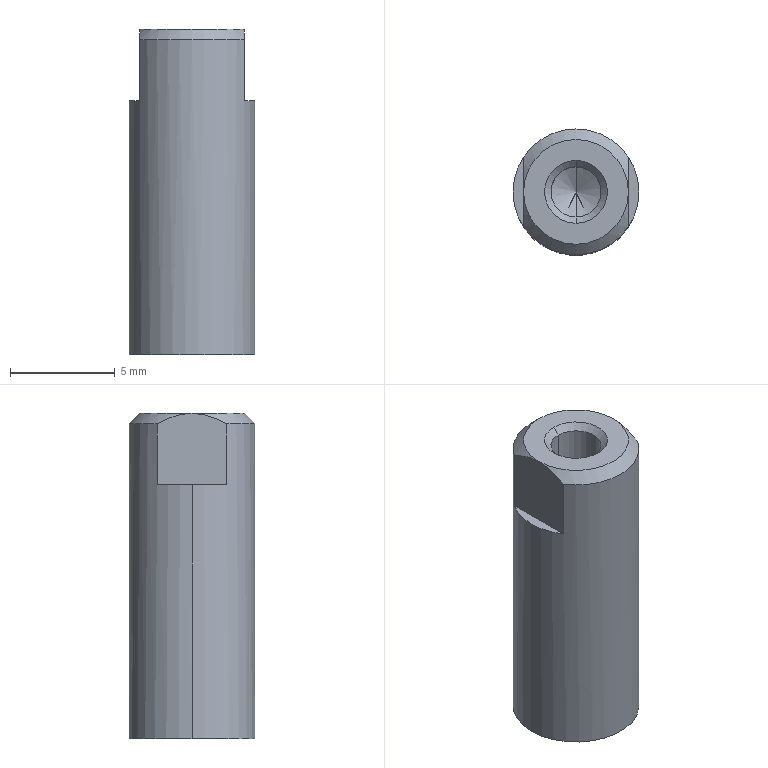Part | STEP file | 4 | 1 solid | 16 faces | box 6 x 6 x 15.5 mm | volume 398.486 mm3 | cone 6 | plane 6 | cylinder 4 | commonest cylinder face diameters 2.39 x2 6 x2
STEP:
#1=CARTESIAN_POINT('',(0.,0.,0.));
#2=DIRECTION('',(0.,0.,1.));
#3=DIRECTION('',(1.,0.,0.));
#4=AXIS2_PLACEMENT_3D('',#1,#2,#3);
#5=CARTESIAN_POINT('',(2.5,1.658,0.1));
#6=VERTEX_POINT('',#5);
#7=CARTESIAN_POINT('',(3.,0.,0.1));
#8=VERTEX_POINT('',#7);
#9=CARTESIAN_POINT('',(0.,0.,0.1));
#10=DIRECTION('',(0.,0.,-1.));
#11=DIRECTION('',(-1.,0.,0.));
#12=AXIS2_PLACEMENT_3D('',#9,#10,#11);
#13=CIRCLE('',#12,3.);
#14=CARTESIAN_POINT('',(0.,0.,-4.5));
#15=DIRECTION('',(0.,0.,-1.));
#16=DIRECTION('',(-1.,0.,0.));
#17=AXIS2_PLACEMENT_3D('',#14,#15,#16);
#18=CYLINDRICAL_SURFACE('',#17,3.);
#19=CARTESIAN_POINT('',(0.,-4.6));
#20=DIRECTION('',(1.,0.));
#21=VECTOR('',#20,1.);
#22=LINE('',#19,#21);
#23=(GEOMETRIC_REPRESENTATION_CONTEXT(2)PARAMETRIC_REPRESENTATION_CONTEXT()REPRESENTATION_CONTEXT('',''));
#24=DEFINITIONAL_REPRESENTATION('',(#22),#23);
#25=PCURVE('',#18,#24);
#26=CARTESIAN_POINT('',(0.,0.,0.1));
#27=DIRECTION('',(0.,0.,1.));
#28=DIRECTION('',(1.,0.,0.));
#29=AXIS2_PLACEMENT_3D('',#26,#27,#28);
#30=PLANE('',#29);
#31=CARTESIAN_POINT('',(-3.,0.));
#32=CARTESIAN_POINT('',(-3.,5.196));
#33=CARTESIAN_POINT('',(1.5,2.598));
#34=CARTESIAN_POINT('',(6.,0.));
#35=CARTESIAN_POINT('',(1.5,-2.598));
#36=CARTESIAN_POINT('',(-3.,-5.196));
#37=CARTESIAN_POINT('',(-3.,0.));
#38=(BOUNDED_CURVE()B_SPLINE_CURVE(2,(#31,#32,#33,#34,#35,#36,#37),.UNSPECIFIED.,.T.,.F.)B_SPLINE_CURVE_WITH_KNOTS((1,2,2,2,2,1),(-2.094,0.,2.094,4.189,6.283,8.378),.UNSPECIFIED.)CURVE()GEOMETRIC_REPRESENTATION_ITEM()RATIONAL_B_SPLINE_CURVE((1.,0.5,1.,0.5,1.,0.5,1.))REPRESENTATION_ITEM(''));
#39=(GEOMETRIC_REPRESENTATION_CONTEXT(2)PARAMETRIC_REPRESENTATION_CONTEXT()REPRESENTATION_CONTEXT('',''));
#40=DEFINITIONAL_REPRESENTATION('',(#38),#39);
#41=PCURVE('',#30,#40);
#42=SURFACE_CURVE('',#13,(#25,#41),.PCURVE_S1.);
#43=EDGE_CURVE('',#6,#8,#42,.T.);
#44=ORIENTED_EDGE('',*,*,#43,.T.);
#45=CARTESIAN_POINT('',(3.,0.,-12.));
#46=VERTEX_POINT('',#45);
#47=CARTESIAN_POINT('',(3.,0.,-4.5));
#48=DIRECTION('',(0.,0.,-1.));
#49=VECTOR('',#48,1.);
#50=LINE('',#47,#49);
#51=CARTESIAN_POINT('',(3.142,0.));
#52=DIRECTION('',(0.,1.));
#53=VECTOR('',#52,1.);
#54=LINE('',#51,#53);
#55=(GEOMETRIC_REPRESENTATION_CONTEXT(2)PARAMETRIC_REPRESENTATION_CONTEXT()REPRESENTATION_CONTEXT('',''));
#56=DEFINITIONAL_REPRESENTATION('',(#54),#55);
#57=PCURVE('',#18,#56);
#58=CARTESIAN_POINT('',(0.,0.,-4.5));
#59=DIRECTION('',(0.,0.,-1.));
#60=DIRECTION('',(-1.,0.,0.));
#61=AXIS2_PLACEMENT_3D('',#58,#59,#60);
#62=CYLINDRICAL_SURFACE('',#61,3.);
#63=CARTESIAN_POINT('',(3.142,0.));
#64=DIRECTION('',(0.,1.));
#65=VECTOR('',#64,1.);
#66=LINE('',#63,#65);
#67=(GEOMETRIC_REPRESENTATION_CONTEXT(2)PARAMETRIC_REPRESENTATION_CONTEXT()REPRESENTATION_CONTEXT('',''));
#68=DEFINITIONAL_REPRESENTATION('',(#66),#67);
#69=PCURVE('',#62,#68);
#70=SURFACE_CURVE('',#50,(#57,#69),.PCURVE_S1.);
#71=EDGE_CURVE('',#8,#46,#70,.T.);
#72=ORIENTED_EDGE('',*,*,#71,.T.);
#73=CARTESIAN_POINT('',(-3.,0.,-12.));
#74=VERTEX_POINT('',#73);
#75=CARTESIAN_POINT('',(0.,0.,-12.));
#76=DIRECTION('',(0.,0.,1.));
#77=DIRECTION('',(-1.,0.,0.));
#78=AXIS2_PLACEMENT_3D('',#75,#76,#77);
#79=CIRCLE('',#78,3.);
#80=CARTESIAN_POINT('',(6.283,7.5));
#81=DIRECTION('',(-1.,0.));
#82=VECTOR('',#81,1.);
#83=LINE('',#80,#82);
#84=(GEOMETRIC_REPRESENTATION_CONTEXT(2)PARAMETRIC_REPRESENTATION_CONTEXT()REPRESENTATION_CONTEXT('',''));
#85=DEFINITIONAL_REPRESENTATION('',(#83),#84);
#86=PCURVE('',#18,#85);
#87=CARTESIAN_POINT('',(0.,1.5,-12.));
#88=DIRECTION('',(0.,0.,-1.));
#89=DIRECTION('',(-1.,0.,0.));
#90=AXIS2_PLACEMENT_3D('',#87,#88,#89);
#91=PLANE('',#90);
#92=CARTESIAN_POINT('',(3.,-1.5));
#93=CARTESIAN_POINT('',(3.,-6.696));
#94=CARTESIAN_POINT('',(-1.5,-4.098));
#95=CARTESIAN_POINT('',(-6.,-1.5));
#96=CARTESIAN_POINT('',(-1.5,1.098));
#97=CARTESIAN_POINT('',(3.,3.696));
#98=CARTESIAN_POINT('',(3.,-1.5));
#99=(BOUNDED_CURVE()B_SPLINE_CURVE(2,(#92,#93,#94,#95,#96,#97,#98),.UNSPECIFIED.,.T.,.F.)B_SPLINE_CURVE_WITH_KNOTS((1,2,2,2,2,1),(-2.094,0.,2.094,4.189,6.283,8.378),.UNSPECIFIED.)CURVE()GEOMETRIC_REPRESENTATION_ITEM()RATIONAL_B_SPLINE_CURVE((1.,0.5,1.,0.5,1.,0.5,1.))REPRESENTATION_ITEM(''));
#100=(GEOMETRIC_REPRESENTATION_CONTEXT(2)PARAMETRIC_REPRESENTATION_CONTEXT()REPRESENTATION_CONTEXT('',''));
#101=DEFINITIONAL_REPRESENTATION('',(#99),#100);
#102=PCURVE('',#91,#101);
#103=SURFACE_CURVE('',#79,(#86,#102),.PCURVE_S1.);
#104=EDGE_CURVE('',#46,#74,#103,.T.);
#105=ORIENTED_EDGE('',*,*,#104,.T.);
#106=CARTESIAN_POINT('',(-3.,0.,0.1));
#107=VERTEX_POINT('',#106);
#108=CARTESIAN_POINT('',(-3.,0.,-4.5));
#109=DIRECTION('',(0.,0.,-1.));
#110=VECTOR('',#109,1.);
#111=LINE('',#108,#110);
#112=CARTESIAN_POINT('',(0.,0.));
#113=DIRECTION('',(0.,1.));
#114=VECTOR('',#113,1.);
#115=LINE('',#112,#114);
#116=(GEOMETRIC_REPRESENTATION_CONTEXT(2)PARAMETRIC_REPRESENTATION_CONTEXT()REPRESENTATION_CONTEXT('',''));
#117=DEFINITIONAL_REPRESENTATION('',(#115),#116);
#118=PCURVE('',#18,#117);
#119=CARTESIAN_POINT('',(6.283,0.));
#120=DIRECTION('',(0.,1.));
#121=VECTOR('',#120,1.);
#122=LINE('',#119,#121);
#123=(GEOMETRIC_REPRESENTATION_CONTEXT(2)PARAMETRIC_REPRESENTATION_CONTEXT()REPRESENTATION_CONTEXT('',''));
#124=DEFINITIONAL_REPRESENTATION('',(#122),#123);
#125=PCURVE('',#62,#124);
#126=SURFACE_CURVE('',#111,(#118,#125),.PCURVE_S1.);
#127=EDGE_CURVE('',#107,#74,#126,.T.);
#128=ORIENTED_EDGE('',*,*,#127,.F.);
#129=CARTESIAN_POINT('',(-2.5,1.658,0.1));
#130=VERTEX_POINT('',#129);
#131=CARTESIAN_POINT('',(0.,0.,0.1));
#132=DIRECTION('',(0.,0.,-1.));
#133=DIRECTION('',(-1.,0.,0.));
#134=AXIS2_PLACEMENT_3D('',#131,#132,#133);
#135=CIRCLE('',#134,3.);
#136=CARTESIAN_POINT('',(0.,-4.6));
#137=DIRECTION('',(1.,0.));
#138=VECTOR('',#137,1.);
#139=LINE('',#136,#138);
#140=(GEOMETRIC_REPRESENTATION_CONTEXT(2)PARAMETRIC_REPRESENTATION_CONTEXT()REPRESENTATION_CONTEXT('',''));
#141=DEFINITIONAL_REPRESENTATION('',(#139),#140);
#142=PCURVE('',#18,#141);
#143=CARTESIAN_POINT('',(0.,0.,0.1));
#144=DIRECTION('',(0.,0.,1.));
#145=DIRECTION('',(1.,0.,0.));
#146=AXIS2_PLACEMENT_3D('',#143,#144,#145);
#147=PLANE('',#146);
#148=CARTESIAN_POINT('',(-3.,0.));
#149=CARTESIAN_POINT('',(-3.,5.196));
#150=CARTESIAN_POINT('',(1.5,2.598));
#151=CARTESIAN_POINT('',(6.,0.));
#152=CARTESIAN_POINT('',(1.5,-2.598));
#153=CARTESIAN_POINT('',(-3.,-5.196));
#154=CARTESIAN_POINT('',(-3.,0.));
#155=(BOUNDED_CURVE()B_SPLINE_CURVE(2,(#148,#149,#150,#151,#152,#153,#154),.UNSPECIFIED.,.T.,.F.)B_SPLINE_CURVE_WITH_KNOTS((1,2,2,2,2,1),(-2.094,0.,2.094,4.189,6.283,8.378),.UNSPECIFIED.)CURVE()GEOMETRIC_REPRESENTATION_ITEM()RATIONAL_B_SPLINE_CURVE((1.,0.5,1.,0.5,1.,0.5,1.))REPRESENTATION_ITEM(''));
#156=(GEOMETRIC_REPRESENTATION_CONTEXT(2)PARAMETRIC_REPRESENTATION_CONTEXT()REPRESENTATION_CONTEXT('',''));
#157=DEFINITIONAL_REPRESENTATION('',(#155),#156);
#158=PCURVE('',#147,#157);
#159=SURFACE_CURVE('',#135,(#142,#158),.PCURVE_S1.);
#160=EDGE_CURVE('',#107,#130,#159,.T.);
#161=ORIENTED_EDGE('',*,*,#160,.T.);
#162=CARTESIAN_POINT('',(-2.5,1.658,3.));
#163=VERTEX_POINT('',#162);
#164=CARTESIAN_POINT('',(-2.5,1.658,-4.5));
#165=DIRECTION('',(0.,0.,1.));
#166=VECTOR('',#165,1.);
#167=LINE('',#164,#166);
#168=CARTESIAN_POINT('',(0.5857,0.));
#169=DIRECTION('',(0.,-1.));
#170=VECTOR('',#169,1.);
#171=LINE('',#168,#170);
#172=(GEOMETRIC_REPRESENTATION_CONTEXT(2)PARAMETRIC_REPRESENTATION_CONTEXT()REPRESENTATION_CONTEXT('',''));
#173=DEFINITIONAL_REPRESENTATION('',(#171),#172);
#174=PCURVE('',#18,#173);
#175=CARTESIAN_POINT('',(-2.5,-5.,3.5));
#176=DIRECTION('',(1.,0.,0.));
#177=DIRECTION('',(0.,0.,-1.));
#178=AXIS2_PLACEMENT_3D('',#175,#176,#177);
#179=PLANE('',#178);
#180=CARTESIAN_POINT('',(8.,6.658));
#181=DIRECTION('',(-1.,0.));
#182=VECTOR('',#181,1.);
#183=LINE('',#180,#182);
#184=(GEOMETRIC_REPRESENTATION_CONTEXT(2)PARAMETRIC_REPRESENTATION_CONTEXT()REPRESENTATION_CONTEXT('',''));
#185=DEFINITIONAL_REPRESENTATION('',(#183),#184);
#186=PCURVE('',#179,#185);
#187=SURFACE_CURVE('',#167,(#174,#186),.PCURVE_S1.);
#188=EDGE_CURVE('',#130,#163,#187,.T.);
#189=ORIENTED_EDGE('',*,*,#188,.T.);
#190=CARTESIAN_POINT('',(2.5,1.658,3.));
#191=VERTEX_POINT('',#190);
#192=CARTESIAN_POINT('',(0.,0.,3.));
#193=DIRECTION('',(0.,0.,-1.));
#194=DIRECTION('',(-1.,0.,0.));
#195=AXIS2_PLACEMENT_3D('',#192,#193,#194);
#196=CIRCLE('',#195,3.);
#197=CARTESIAN_POINT('',(0.,-7.5));
#198=DIRECTION('',(1.,0.));
#199=VECTOR('',#198,1.);
#200=LINE('',#197,#199);
#201=(GEOMETRIC_REPRESENTATION_CONTEXT(2)PARAMETRIC_REPRESENTATION_CONTEXT()REPRESENTATION_CONTEXT('',''));
#202=DEFINITIONAL_REPRESENTATION('',(#200),#201);
#203=PCURVE('',#18,#202);
#204=CARTESIAN_POINT('',(0.,0.,3.));
#205=DIRECTION('',(0.,0.,-1.));
#206=DIRECTION('',(-1.,0.,0.));
#207=AXIS2_PLACEMENT_3D('',#204,#205,#206);
#208=CONICAL_SURFACE('',#207,3.,0.7854);
#209=CARTESIAN_POINT('',(0.,0.));
#210=DIRECTION('',(1.,0.));
#211=VECTOR('',#210,1.);
#212=LINE('',#209,#211);
#213=(GEOMETRIC_REPRESENTATION_CONTEXT(2)PARAMETRIC_REPRESENTATION_CONTEXT()REPRESENTATION_CONTEXT('',''));
#214=DEFINITIONAL_REPRESENTATION('',(#212),#213);
#215=PCURVE('',#208,#214);
#216=SURFACE_CURVE('',#196,(#203,#215),.PCURVE_S1.);
#217=EDGE_CURVE('',#163,#191,#216,.T.);
#218=ORIENTED_EDGE('',*,*,#217,.T.);
#219=CARTESIAN_POINT('',(2.5,1.658,-4.5));
#220=DIRECTION('',(0.,0.,-1.));
#221=VECTOR('',#220,1.);
#222=LINE('',#219,#221);
#223=CARTESIAN_POINT('',(2.556,0.));
#224=DIRECTION('',(0.,1.));
#225=VECTOR('',#224,1.);
#226=LINE('',#223,#225);
#227=(GEOMETRIC_REPRESENTATION_CONTEXT(2)PARAMETRIC_REPRESENTATION_CONTEXT()REPRESENTATION_CONTEXT('',''));
#228=DEFINITIONAL_REPRESENTATION('',(#226),#227);
#229=PCURVE('',#18,#228);
#230=CARTESIAN_POINT('',(2.5,5.,3.5));
#231=DIRECTION('',(-1.,0.,0.));
#232=DIRECTION('',(0.,0.,1.));
#233=AXIS2_PLACEMENT_3D('',#230,#231,#232);
#234=PLANE('',#233);
#235=CARTESIAN_POINT('',(-8.,-3.342));
#236=DIRECTION('',(-1.,0.));
#237=VECTOR('',#236,1.);
#238=LINE('',#235,#237);
#239=(GEOMETRIC_REPRESENTATION_CONTEXT(2)PARAMETRIC_REPRESENTATION_CONTEXT()REPRESENTATION_CONTEXT('',''));
#240=DEFINITIONAL_REPRESENTATION('',(#238),#239);
#241=PCURVE('',#234,#240);
#242=SURFACE_CURVE('',#222,(#229,#241),.PCURVE_S1.);
#243=EDGE_CURVE('',#191,#6,#242,.T.);
#244=ORIENTED_EDGE('',*,*,#243,.T.);
#245=EDGE_LOOP('',(#44,#72,#105,#128,#161,#189,#218,#244));
#246=FACE_BOUND('',#245,.T.);
#247=ADVANCED_FACE('',(#246),#18,.T.);
#248=CARTESIAN_POINT('',(0.,-1.195,3.195));
#249=VERTEX_POINT('',#248);
#250=CARTESIAN_POINT('',(0.,-1.5,3.5));
#251=VERTEX_POINT('',#250);
#252=CARTESIAN_POINT('',(0.,-1.5,3.5));
#253=DIRECTION('',(0.,-0.7071,0.7071));
#254=VECTOR('',#253,1.);
#255=LINE('',#252,#254);
#256=CARTESIAN_POINT('',(0.,0.,3.5));
#257=DIRECTION('',(0.,0.,1.));
#258=DIRECTION('',(0.,-1.,0.));
#259=AXIS2_PLACEMENT_3D('',#256,#257,#258);
#260=CONICAL_SURFACE('',#259,1.5,0.7854);
#261=CARTESIAN_POINT('',(6.283,0.));
#262=DIRECTION('',(0.,1.));
#263=VECTOR('',#262,1.);
#264=LINE('',#261,#263);
#265=(GEOMETRIC_REPRESENTATION_CONTEXT(2)PARAMETRIC_REPRESENTATION_CONTEXT()REPRESENTATION_CONTEXT('',''));
#266=DEFINITIONAL_REPRESENTATION('',(#264),#265);
#267=PCURVE('',#260,#266);
#268=CARTESIAN_POINT('',(0.,0.,3.5));
#269=DIRECTION('',(0.,0.,1.));
#270=DIRECTION('',(0.,-1.,0.));
#271=AXIS2_PLACEMENT_3D('',#268,#269,#270);
#272=CONICAL_SURFACE('',#271,1.5,0.7854);
#273=CARTESIAN_POINT('',(0.,0.));
#274=DIRECTION('',(0.,1.));
#275=VECTOR('',#274,1.);
#276=LINE('',#273,#275);
#277=(GEOMETRIC_REPRESENTATION_CONTEXT(2)PARAMETRIC_REPRESENTATION_CONTEXT()REPRESENTATION_CONTEXT('',''));
#278=DEFINITIONAL_REPRESENTATION('',(#276),#277);
#279=PCURVE('',#272,#278);
#280=SURFACE_CURVE('',#255,(#267,#279),.PCURVE_S1.);
#281=EDGE_CURVE('',#249,#251,#280,.T.);
#282=ORIENTED_EDGE('',*,*,#281,.T.);
#283=CARTESIAN_POINT('',(0.,1.5,3.5));
#284=VERTEX_POINT('',#283);
#285=CARTESIAN_POINT('',(0.,0.,3.5));
#286=DIRECTION('',(0.,0.,-1.));
#287=DIRECTION('',(0.,-1.,0.));
#288=AXIS2_PLACEMENT_3D('',#285,#286,#287);
#289=CIRCLE('',#288,1.5);
#290=CARTESIAN_POINT('',(6.283,0.));
#291=DIRECTION('',(-1.,0.));
#292=VECTOR('',#291,1.);
#293=LINE('',#290,#292);
#294=(GEOMETRIC_REPRESENTATION_CONTEXT(2)PARAMETRIC_REPRESENTATION_CONTEXT()REPRESENTATION_CONTEXT('',''));
#295=DEFINITIONAL_REPRESENTATION('',(#293),#294);
#296=PCURVE('',#260,#295);
#297=CARTESIAN_POINT('',(0.,1.25,3.5));
#298=DIRECTION('',(0.,0.,1.));
#299=DIRECTION('',(1.,0.,0.));
#300=AXIS2_PLACEMENT_3D('',#297,#298,#299);
#301=PLANE('',#300);
#302=CARTESIAN_POINT('',(0.,-2.75));
#303=CARTESIAN_POINT('',(-2.598,-2.75));
#304=CARTESIAN_POINT('',(-1.299,-0.5));
#305=CARTESIAN_POINT('',(0.,1.75));
#306=CARTESIAN_POINT('',(1.299,-0.5));
#307=CARTESIAN_POINT('',(2.598,-2.75));
#308=CARTESIAN_POINT('',(0.,-2.75));
#309=(BOUNDED_CURVE()B_SPLINE_CURVE(2,(#302,#303,#304,#305,#306,#307,#308),.UNSPECIFIED.,.T.,.F.)B_SPLINE_CURVE_WITH_KNOTS((1,2,2,2,2,1),(-2.094,0.,2.094,4.189,6.283,8.378),.UNSPECIFIED.)CURVE()GEOMETRIC_REPRESENTATION_ITEM()RATIONAL_B_SPLINE_CURVE((1.,0.5,1.,0.5,1.,0.5,1.))REPRESENTATION_ITEM(''));
#310=(GEOMETRIC_REPRESENTATION_CONTEXT(2)PARAMETRIC_REPRESENTATION_CONTEXT()REPRESENTATION_CONTEXT('',''));
#311=DEFINITIONAL_REPRESENTATION('',(#309),#310);
#312=PCURVE('',#301,#311);
#313=SURFACE_CURVE('',#289,(#296,#312),.PCURVE_S1.);
#314=EDGE_CURVE('',#251,#284,#313,.T.);
#315=ORIENTED_EDGE('',*,*,#314,.T.);
#316=CARTESIAN_POINT('',(0.,1.195,3.195));
#317=VERTEX_POINT('',#316);
#318=CARTESIAN_POINT('',(0.,1.5,3.5));
#319=DIRECTION('',(0.,0.7071,0.7071));
#320=VECTOR('',#319,1.);
#321=LINE('',#318,#320);
#322=CARTESIAN_POINT('',(3.142,0.));
#323=DIRECTION('',(0.,1.));
#324=VECTOR('',#323,1.);
#325=LINE('',#322,#324);
#326=(GEOMETRIC_REPRESENTATION_CONTEXT(2)PARAMETRIC_REPRESENTATION_CONTEXT()REPRESENTATION_CONTEXT('',''));
#327=DEFINITIONAL_REPRESENTATION('',(#325),#326);
#328=PCURVE('',#260,#327);
#329=CARTESIAN_POINT('',(3.142,0.));
#330=DIRECTION('',(0.,1.));
#331=VECTOR('',#330,1.);
#332=LINE('',#329,#331);
#333=(GEOMETRIC_REPRESENTATION_CONTEXT(2)PARAMETRIC_REPRESENTATION_CONTEXT()REPRESENTATION_CONTEXT('',''));
#334=DEFINITIONAL_REPRESENTATION('',(#332),#333);
#335=PCURVE('',#272,#334);
#336=SURFACE_CURVE('',#321,(#328,#335),.PCURVE_S1.);
#337=EDGE_CURVE('',#317,#284,#336,.T.);
#338=ORIENTED_EDGE('',*,*,#337,.F.);
#339=CARTESIAN_POINT('',(0.,0.,3.195));
#340=DIRECTION('',(0.,0.,1.));
#341=DIRECTION('',(0.,1.,0.));
#342=AXIS2_PLACEMENT_3D('',#339,#340,#341);
#343=CIRCLE('',#342,1.195);
#344=CARTESIAN_POINT('',(3.142,-0.305));
#345=DIRECTION('',(1.,0.));
#346=VECTOR('',#345,1.);
#347=LINE('',#344,#346);
#348=(GEOMETRIC_REPRESENTATION_CONTEXT(2)PARAMETRIC_REPRESENTATION_CONTEXT()REPRESENTATION_CONTEXT('',''));
#349=DEFINITIONAL_REPRESENTATION('',(#347),#348);
#350=PCURVE('',#260,#349);
#351=CARTESIAN_POINT('',(0.,0.,0.0975));
#352=DIRECTION('',(0.,0.,-1.));
#353=DIRECTION('',(0.,1.,0.));
#354=AXIS2_PLACEMENT_3D('',#351,#352,#353);
#355=CYLINDRICAL_SURFACE('',#354,1.195);
#356=CARTESIAN_POINT('',(6.283,-3.098));
#357=DIRECTION('',(-1.,0.));
#358=VECTOR('',#357,1.);
#359=LINE('',#356,#358);
#360=(GEOMETRIC_REPRESENTATION_CONTEXT(2)PARAMETRIC_REPRESENTATION_CONTEXT()REPRESENTATION_CONTEXT('',''));
#361=DEFINITIONAL_REPRESENTATION('',(#359),#360);
#362=PCURVE('',#355,#361);
#363=SURFACE_CURVE('',#343,(#350,#362),.PCURVE_S1.);
#364=EDGE_CURVE('',#317,#249,#363,.T.);
#365=ORIENTED_EDGE('',*,*,#364,.T.);
#366=EDGE_LOOP('',(#282,#315,#338,#365));
#367=FACE_BOUND('',#366,.F.);
#368=ADVANCED_FACE('',(#367),#260,.F.);
#369=CARTESIAN_POINT('',(0.,1.195,-3.));
#370=VERTEX_POINT('',#369);
#371=CARTESIAN_POINT('',(0.,1.195,0.0975));
#372=DIRECTION('',(0.,0.,-1.));
#373=VECTOR('',#372,1.);
#374=LINE('',#371,#373);
#375=CARTESIAN_POINT('',(6.283,0.));
#376=DIRECTION('',(0.,1.));
#377=VECTOR('',#376,1.);
#378=LINE('',#375,#377);
#379=(GEOMETRIC_REPRESENTATION_CONTEXT(2)PARAMETRIC_REPRESENTATION_CONTEXT()REPRESENTATION_CONTEXT('',''));
#380=DEFINITIONAL_REPRESENTATION('',(#378),#379);
#381=PCURVE('',#355,#380);
#382=CARTESIAN_POINT('',(0.,0.,0.0975));
#383=DIRECTION('',(0.,0.,-1.));
#384=DIRECTION('',(0.,1.,0.));
#385=AXIS2_PLACEMENT_3D('',#382,#383,#384);
#386=CYLINDRICAL_SURFACE('',#385,1.195);
#387=CARTESIAN_POINT('',(0.,0.));
#388=DIRECTION('',(0.,1.));
#389=VECTOR('',#388,1.);
#390=LINE('',#387,#389);
#391=(GEOMETRIC_REPRESENTATION_CONTEXT(2)PARAMETRIC_REPRESENTATION_CONTEXT()REPRESENTATION_CONTEXT('',''));
#392=DEFINITIONAL_REPRESENTATION('',(#390),#391);
#393=PCURVE('',#386,#392);
#394=SURFACE_CURVE('',#374,(#381,#393),.PCURVE_S1.);
#395=EDGE_CURVE('',#317,#370,#394,.T.);
#396=ORIENTED_EDGE('',*,*,#395,.T.);
#397=CARTESIAN_POINT('',(0.,-1.195,-3.));
#398=VERTEX_POINT('',#397);
#399=CARTESIAN_POINT('',(0.,0.,-3.));
#400=DIRECTION('',(0.,0.,1.));
#401=DIRECTION('',(0.,1.,0.));
#402=AXIS2_PLACEMENT_3D('',#399,#400,#401);
#403=CIRCLE('',#402,1.195);
#404=CARTESIAN_POINT('',(6.283,3.098));
#405=DIRECTION('',(-1.,0.));
#406=VECTOR('',#405,1.);
#407=LINE('',#404,#406);
#408=(GEOMETRIC_REPRESENTATION_CONTEXT(2)PARAMETRIC_REPRESENTATION_CONTEXT()REPRESENTATION_CONTEXT('',''));
#409=DEFINITIONAL_REPRESENTATION('',(#407),#408);
#410=PCURVE('',#355,#409);
#411=CARTESIAN_POINT('',(0.,0.,-3.));
#412=DIRECTION('',(0.,0.,1.));
#413=DIRECTION('',(0.,-1.,0.));
#414=AXIS2_PLACEMENT_3D('',#411,#412,#413);
#415=CONICAL_SURFACE('',#414,1.195,1.047);
#416=CARTESIAN_POINT('',(3.142,0.));
#417=DIRECTION('',(1.,0.));
#418=VECTOR('',#417,1.);
#419=LINE('',#416,#418);
#420=(GEOMETRIC_REPRESENTATION_CONTEXT(2)PARAMETRIC_REPRESENTATION_CONTEXT()REPRESENTATION_CONTEXT('',''));
#421=DEFINITIONAL_REPRESENTATION('',(#419),#420);
#422=PCURVE('',#415,#421);
#423=SURFACE_CURVE('',#403,(#410,#422),.PCURVE_S1.);
#424=EDGE_CURVE('',#370,#398,#423,.T.);
#425=ORIENTED_EDGE('',*,*,#424,.T.);
#426=CARTESIAN_POINT('',(0.,-1.195,0.0975));
#427=DIRECTION('',(0.,0.,-1.));
#428=VECTOR('',#427,1.);
#429=LINE('',#426,#428);
#430=CARTESIAN_POINT('',(3.142,0.));
#431=DIRECTION('',(0.,1.));
#432=VECTOR('',#431,1.);
#433=LINE('',#430,#432);
#434=(GEOMETRIC_REPRESENTATION_CONTEXT(2)PARAMETRIC_REPRESENTATION_CONTEXT()REPRESENTATION_CONTEXT('',''));
#435=DEFINITIONAL_REPRESENTATION('',(#433),#434);
#436=PCURVE('',#355,#435);
#437=CARTESIAN_POINT('',(3.142,0.));
#438=DIRECTION('',(0.,1.));
#439=VECTOR('',#438,1.);
#440=LINE('',#437,#439);
#441=(GEOMETRIC_REPRESENTATION_CONTEXT(2)PARAMETRIC_REPRESENTATION_CONTEXT()REPRESENTATION_CONTEXT('',''));
#442=DEFINITIONAL_REPRESENTATION('',(#440),#441);
#443=PCURVE('',#386,#442);
#444=SURFACE_CURVE('',#429,(#436,#443),.PCURVE_S1.);
#445=EDGE_CURVE('',#249,#398,#444,.T.);
#446=ORIENTED_EDGE('',*,*,#445,.F.);
#447=ORIENTED_EDGE('',*,*,#364,.F.);
#448=EDGE_LOOP('',(#396,#425,#446,#447));
#449=FACE_BOUND('',#448,.F.);
#450=ADVANCED_FACE('',(#449),#355,.F.);
#451=ORIENTED_EDGE('',*,*,#424,.F.);
#452=CARTESIAN_POINT('',(0.,0.,-3.69));
#453=VERTEX_POINT('',#452);
#454=CARTESIAN_POINT('',(0.,1.195,-3.));
#455=DIRECTION('',(0.,0.866,0.5));
#456=VECTOR('',#455,1.);
#457=LINE('',#454,#456);
#458=CARTESIAN_POINT('',(3.142,0.));
#459=DIRECTION('',(0.,1.));
#460=VECTOR('',#459,1.);
#461=LINE('',#458,#460);
#462=(GEOMETRIC_REPRESENTATION_CONTEXT(2)PARAMETRIC_REPRESENTATION_CONTEXT()REPRESENTATION_CONTEXT('',''));
#463=DEFINITIONAL_REPRESENTATION('',(#461),#462);
#464=PCURVE('',#415,#463);
#465=CARTESIAN_POINT('',(0.,0.,-3.));
#466=DIRECTION('',(0.,0.,1.));
#467=DIRECTION('',(0.,-1.,0.));
#468=AXIS2_PLACEMENT_3D('',#465,#466,#467);
#469=CONICAL_SURFACE('',#468,1.195,1.047);
#470=CARTESIAN_POINT('',(3.142,0.));
#471=DIRECTION('',(0.,1.));
#472=VECTOR('',#471,1.);
#473=LINE('',#470,#472);
#474=(GEOMETRIC_REPRESENTATION_CONTEXT(2)PARAMETRIC_REPRESENTATION_CONTEXT()REPRESENTATION_CONTEXT('',''));
#475=DEFINITIONAL_REPRESENTATION('',(#473),#474);
#476=PCURVE('',#469,#475);
#477=SURFACE_CURVE('',#457,(#464,#476),.PCURVE_S1.);
#478=EDGE_CURVE('',#453,#370,#477,.T.);
#479=ORIENTED_EDGE('',*,*,#478,.F.);
#480=CARTESIAN_POINT('',(0.,-1.195,-3.));
#481=DIRECTION('',(0.,-0.866,0.5));
#482=VECTOR('',#481,1.);
#483=LINE('',#480,#482);
#484=CARTESIAN_POINT('',(6.283,0.));
#485=DIRECTION('',(0.,1.));
#486=VECTOR('',#485,1.);
#487=LINE('',#484,#486);
#488=(GEOMETRIC_REPRESENTATION_CONTEXT(2)PARAMETRIC_REPRESENTATION_CONTEXT()REPRESENTATION_CONTEXT('',''));
#489=DEFINITIONAL_REPRESENTATION('',(#487),#488);
#490=PCURVE('',#415,#489);
#491=CARTESIAN_POINT('',(0.,0.));
#492=DIRECTION('',(0.,1.));
#493=VECTOR('',#492,1.);
#494=LINE('',#491,#493);
#495=(GEOMETRIC_REPRESENTATION_CONTEXT(2)PARAMETRIC_REPRESENTATION_CONTEXT()REPRESENTATION_CONTEXT('',''));
#496=DEFINITIONAL_REPRESENTATION('',(#494),#495);
#497=PCURVE('',#469,#496);
#498=SURFACE_CURVE('',#483,(#490,#497),.PCURVE_S1.);
#499=EDGE_CURVE('',#453,#398,#498,.T.);
#500=ORIENTED_EDGE('',*,*,#499,.T.);
#501=EDGE_LOOP('',(#451,#479,#500));
#502=FACE_BOUND('',#501,.F.);
#503=ADVANCED_FACE('',(#502),#415,.F.);
#504=ORIENTED_EDGE('',*,*,#71,.F.);
#505=CARTESIAN_POINT('',(2.5,-1.658,0.1));
#506=VERTEX_POINT('',#505);
#507=CARTESIAN_POINT('',(0.,0.,0.1));
#508=DIRECTION('',(0.,0.,-1.));
#509=DIRECTION('',(-1.,0.,0.));
#510=AXIS2_PLACEMENT_3D('',#507,#508,#509);
#511=CIRCLE('',#510,3.);
#512=CARTESIAN_POINT('',(0.,-4.6));
#513=DIRECTION('',(1.,0.));
#514=VECTOR('',#513,1.);
#515=LINE('',#512,#514);
#516=(GEOMETRIC_REPRESENTATION_CONTEXT(2)PARAMETRIC_REPRESENTATION_CONTEXT()REPRESENTATION_CONTEXT('',''));
#517=DEFINITIONAL_REPRESENTATION('',(#515),#516);
#518=PCURVE('',#62,#517);
#519=CARTESIAN_POINT('',(-3.,0.));
#520=CARTESIAN_POINT('',(-3.,5.196));
#521=CARTESIAN_POINT('',(1.5,2.598));
#522=CARTESIAN_POINT('',(6.,0.));
#523=CARTESIAN_POINT('',(1.5,-2.598));
#524=CARTESIAN_POINT('',(-3.,-5.196));
#525=CARTESIAN_POINT('',(-3.,0.));
#526=(BOUNDED_CURVE()B_SPLINE_CURVE(2,(#519,#520,#521,#522,#523,#524,#525),.UNSPECIFIED.,.T.,.F.)B_SPLINE_CURVE_WITH_KNOTS((1,2,2,2,2,1),(-2.094,0.,2.094,4.189,6.283,8.378),.UNSPECIFIED.)CURVE()GEOMETRIC_REPRESENTATION_ITEM()RATIONAL_B_SPLINE_CURVE((1.,0.5,1.,0.5,1.,0.5,1.))REPRESENTATION_ITEM(''));
#527=(GEOMETRIC_REPRESENTATION_CONTEXT(2)PARAMETRIC_REPRESENTATION_CONTEXT()REPRESENTATION_CONTEXT('',''));
#528=DEFINITIONAL_REPRESENTATION('',(#526),#527);
#529=PCURVE('',#30,#528);
#530=SURFACE_CURVE('',#511,(#518,#529),.PCURVE_S1.);
#531=EDGE_CURVE('',#8,#506,#530,.T.);
#532=ORIENTED_EDGE('',*,*,#531,.T.);
#533=CARTESIAN_POINT('',(2.5,-1.658,3.));
#534=VERTEX_POINT('',#533);
#535=CARTESIAN_POINT('',(2.5,-1.658,-4.5));
#536=DIRECTION('',(0.,0.,1.));
#537=VECTOR('',#536,1.);
#538=LINE('',#535,#537);
#539=CARTESIAN_POINT('',(3.727,0.));
#540=DIRECTION('',(0.,-1.));
#541=VECTOR('',#540,1.);
#542=LINE('',#539,#541);
#543=(GEOMETRIC_REPRESENTATION_CONTEXT(2)PARAMETRIC_REPRESENTATION_CONTEXT()REPRESENTATION_CONTEXT('',''));
#544=DEFINITIONAL_REPRESENTATION('',(#542),#543);
#545=PCURVE('',#62,#544);
#546=CARTESIAN_POINT('',(-8.,-6.658));
#547=DIRECTION('',(1.,0.));
#548=VECTOR('',#547,1.);
#549=LINE('',#546,#548);
#550=(GEOMETRIC_REPRESENTATION_CONTEXT(2)PARAMETRIC_REPRESENTATION_CONTEXT()REPRESENTATION_CONTEXT('',''));
#551=DEFINITIONAL_REPRESENTATION('',(#549),#550);
#552=PCURVE('',#234,#551);
#553=SURFACE_CURVE('',#538,(#545,#552),.PCURVE_S1.);
#554=EDGE_CURVE('',#506,#534,#553,.T.);
#555=ORIENTED_EDGE('',*,*,#554,.T.);
#556=CARTESIAN_POINT('',(-2.5,-1.658,3.));
#557=VERTEX_POINT('',#556);
#558=CARTESIAN_POINT('',(0.,0.,3.));
#559=DIRECTION('',(0.,0.,-1.));
#560=DIRECTION('',(-1.,0.,0.));
#561=AXIS2_PLACEMENT_3D('',#558,#559,#560);
#562=CIRCLE('',#561,3.);
#563=CARTESIAN_POINT('',(0.,-7.5));
#564=DIRECTION('',(1.,0.));
#565=VECTOR('',#564,1.);
#566=LINE('',#563,#565);
#567=(GEOMETRIC_REPRESENTATION_CONTEXT(2)PARAMETRIC_REPRESENTATION_CONTEXT()REPRESENTATION_CONTEXT('',''));
#568=DEFINITIONAL_REPRESENTATION('',(#566),#567);
#569=PCURVE('',#62,#568);
#570=CARTESIAN_POINT('',(0.,0.,3.));
#571=DIRECTION('',(0.,0.,-1.));
#572=DIRECTION('',(-1.,0.,0.));
#573=AXIS2_PLACEMENT_3D('',#570,#571,#572);
#574=CONICAL_SURFACE('',#573,3.,0.7854);
#575=CARTESIAN_POINT('',(0.,0.));
#576=DIRECTION('',(1.,0.));
#577=VECTOR('',#576,1.);
#578=LINE('',#575,#577);
#579=(GEOMETRIC_REPRESENTATION_CONTEXT(2)PARAMETRIC_REPRESENTATION_CONTEXT()REPRESENTATION_CONTEXT('',''));
#580=DEFINITIONAL_REPRESENTATION('',(#578),#579);
#581=PCURVE('',#574,#580);
#582=SURFACE_CURVE('',#562,(#569,#581),.PCURVE_S1.);
#583=EDGE_CURVE('',#534,#557,#582,.T.);
#584=ORIENTED_EDGE('',*,*,#583,.T.);
#585=CARTESIAN_POINT('',(-2.5,-1.658,0.1));
#586=VERTEX_POINT('',#585);
#587=CARTESIAN_POINT('',(-2.5,-1.658,-4.5));
#588=DIRECTION('',(0.,0.,-1.));
#589=VECTOR('',#588,1.);
#590=LINE('',#587,#589);
#591=CARTESIAN_POINT('',(5.697,0.));
#592=DIRECTION('',(0.,1.));
#593=VECTOR('',#592,1.);
#594=LINE('',#591,#593);
#595=(GEOMETRIC_REPRESENTATION_CONTEXT(2)PARAMETRIC_REPRESENTATION_CONTEXT()REPRESENTATION_CONTEXT('',''));
#596=DEFINITIONAL_REPRESENTATION('',(#594),#595);
#597=PCURVE('',#62,#596);
#598=CARTESIAN_POINT('',(8.,3.342));
#599=DIRECTION('',(1.,0.));
#600=VECTOR('',#599,1.);
#601=LINE('',#598,#600);
#602=(GEOMETRIC_REPRESENTATION_CONTEXT(2)PARAMETRIC_REPRESENTATION_CONTEXT()REPRESENTATION_CONTEXT('',''));
#603=DEFINITIONAL_REPRESENTATION('',(#601),#602);
#604=PCURVE('',#179,#603);
#605=SURFACE_CURVE('',#590,(#597,#604),.PCURVE_S1.);
#606=EDGE_CURVE('',#557,#586,#605,.T.);
#607=ORIENTED_EDGE('',*,*,#606,.T.);
#608=CARTESIAN_POINT('',(0.,0.,0.1));
#609=DIRECTION('',(0.,0.,-1.));
#610=DIRECTION('',(-1.,0.,0.));
#611=AXIS2_PLACEMENT_3D('',#608,#609,#610);
#612=CIRCLE('',#611,3.);
#613=CARTESIAN_POINT('',(0.,-4.6));
#614=DIRECTION('',(1.,0.));
#615=VECTOR('',#614,1.);
#616=LINE('',#613,#615);
#617=(GEOMETRIC_REPRESENTATION_CONTEXT(2)PARAMETRIC_REPRESENTATION_CONTEXT()REPRESENTATION_CONTEXT('',''));
#618=DEFINITIONAL_REPRESENTATION('',(#616),#617);
#619=PCURVE('',#62,#618);
#620=CARTESIAN_POINT('',(-3.,0.));
#621=CARTESIAN_POINT('',(-3.,5.196));
#622=CARTESIAN_POINT('',(1.5,2.598));
#623=CARTESIAN_POINT('',(6.,0.));
#624=CARTESIAN_POINT('',(1.5,-2.598));
#625=CARTESIAN_POINT('',(-3.,-5.196));
#626=CARTESIAN_POINT('',(-3.,0.));
#627=(BOUNDED_CURVE()B_SPLINE_CURVE(2,(#620,#621,#622,#623,#624,#625,#626),.UNSPECIFIED.,.T.,.F.)B_SPLINE_CURVE_WITH_KNOTS((1,2,2,2,2,1),(-2.094,0.,2.094,4.189,6.283,8.378),.UNSPECIFIED.)CURVE()GEOMETRIC_REPRESENTATION_ITEM()RATIONAL_B_SPLINE_CURVE((1.,0.5,1.,0.5,1.,0.5,1.))REPRESENTATION_ITEM(''));
#628=(GEOMETRIC_REPRESENTATION_CONTEXT(2)PARAMETRIC_REPRESENTATION_CONTEXT()REPRESENTATION_CONTEXT('',''));
#629=DEFINITIONAL_REPRESENTATION('',(#627),#628);
#630=PCURVE('',#147,#629);
#631=SURFACE_CURVE('',#612,(#619,#630),.PCURVE_S1.);
#632=EDGE_CURVE('',#586,#107,#631,.T.);
#633=ORIENTED_EDGE('',*,*,#632,.T.);
#634=ORIENTED_EDGE('',*,*,#127,.T.);
#635=CARTESIAN_POINT('',(0.,0.,-12.));
#636=DIRECTION('',(0.,0.,1.));
#637=DIRECTION('',(-1.,0.,0.));
#638=AXIS2_PLACEMENT_3D('',#635,#636,#637);
#639=CIRCLE('',#638,3.);
#640=CARTESIAN_POINT('',(6.283,7.5));
#641=DIRECTION('',(-1.,0.));
#642=VECTOR('',#641,1.);
#643=LINE('',#640,#642);
#644=(GEOMETRIC_REPRESENTATION_CONTEXT(2)PARAMETRIC_REPRESENTATION_CONTEXT()REPRESENTATION_CONTEXT('',''));
#645=DEFINITIONAL_REPRESENTATION('',(#643),#644);
#646=PCURVE('',#62,#645);
#647=CARTESIAN_POINT('',(3.,-1.5));
#648=CARTESIAN_POINT('',(3.,-6.696));
#649=CARTESIAN_POINT('',(-1.5,-4.098));
#650=CARTESIAN_POINT('',(-6.,-1.5));
#651=CARTESIAN_POINT('',(-1.5,1.098));
#652=CARTESIAN_POINT('',(3.,3.696));
#653=CARTESIAN_POINT('',(3.,-1.5));
#654=(BOUNDED_CURVE()B_SPLINE_CURVE(2,(#647,#648,#649,#650,#651,#652,#653),.UNSPECIFIED.,.T.,.F.)B_SPLINE_CURVE_WITH_KNOTS((1,2,2,2,2,1),(-2.094,0.,2.094,4.189,6.283,8.378),.UNSPECIFIED.)CURVE()GEOMETRIC_REPRESENTATION_ITEM()RATIONAL_B_SPLINE_CURVE((1.,0.5,1.,0.5,1.,0.5,1.))REPRESENTATION_ITEM(''));
#655=(GEOMETRIC_REPRESENTATION_CONTEXT(2)PARAMETRIC_REPRESENTATION_CONTEXT()REPRESENTATION_CONTEXT('',''));
#656=DEFINITIONAL_REPRESENTATION('',(#654),#655);
#657=PCURVE('',#91,#656);
#658=SURFACE_CURVE('',#639,(#646,#657),.PCURVE_S1.);
#659=EDGE_CURVE('',#74,#46,#658,.T.);
#660=ORIENTED_EDGE('',*,*,#659,.T.);
#661=EDGE_LOOP('',(#504,#532,#555,#584,#607,#633,#634,#660));
#662=FACE_BOUND('',#661,.T.);
#663=ADVANCED_FACE('',(#662),#62,.T.);
#664=ORIENTED_EDGE('',*,*,#659,.F.);
#665=ORIENTED_EDGE('',*,*,#104,.F.);
#666=EDGE_LOOP('',(#664,#665));
#667=FACE_BOUND('',#666,.T.);
#668=ADVANCED_FACE('',(#667),#91,.T.);
#669=CARTESIAN_POINT('',(2.5,0.,3.5));
#670=VERTEX_POINT('',#669);
#671=CARTESIAN_POINT('',(2.5,-1.658,3.));
#672=CARTESIAN_POINT('',(2.5,-1.402,3.142));
#673=CARTESIAN_POINT('',(2.5,-1.139,3.265));
#674=CARTESIAN_POINT('',(2.5,-0.5868,3.445));
#675=CARTESIAN_POINT('',(2.5,-0.2946,3.5));
#676=CARTESIAN_POINT('',(2.5,0.,3.5));
#677=B_SPLINE_CURVE_WITH_KNOTS('',3,(#671,#672,#673,#674,#675,#676),.UNSPECIFIED.,.F.,.F.,(4,2,4),(0.,0.0008701,0.00174),.UNSPECIFIED.);
#678=CARTESIAN_POINT('',(3.727,0.));
#679=CARTESIAN_POINT('',(3.721,-0.01287));
#680=CARTESIAN_POINT('',(3.708,-0.03829));
#681=CARTESIAN_POINT('',(3.687,-0.07547));
#682=CARTESIAN_POINT('',(3.666,-0.1116));
#683=CARTESIAN_POINT('',(3.645,-0.1466));
#684=CARTESIAN_POINT('',(3.623,-0.1805));
#685=CARTESIAN_POINT('',(3.6,-0.2132));
#686=CARTESIAN_POINT('',(3.576,-0.2445));
#687=CARTESIAN_POINT('',(3.552,-0.2745));
#688=CARTESIAN_POINT('',(3.526,-0.3031));
#689=CARTESIAN_POINT('',(3.501,-0.3301));
#690=CARTESIAN_POINT('',(3.474,-0.3555));
#691=CARTESIAN_POINT('',(3.447,-0.3792));
#692=CARTESIAN_POINT('',(3.419,-0.4011));
#693=CARTESIAN_POINT('',(3.39,-0.4211));
#694=CARTESIAN_POINT('',(3.361,-0.4391));
#695=CARTESIAN_POINT('',(3.33,-0.4549));
#696=CARTESIAN_POINT('',(3.3,-0.4685));
#697=CARTESIAN_POINT('',(3.269,-0.4798));
#698=CARTESIAN_POINT('',(3.237,-0.4888));
#699=CARTESIAN_POINT('',(3.206,-0.4952));
#700=CARTESIAN_POINT('',(3.174,-0.4991));
#701=CARTESIAN_POINT('',(3.152,-0.5));
#702=CARTESIAN_POINT('',(3.142,-0.5));
#703=B_SPLINE_CURVE_WITH_KNOTS('',3,(#678,#679,#680,#681,#682,#683,#684,#685,#686,#687,#688,#689,#690,#691,#692,#693,#694,#695,#696,#697,#698,#699,#700,#701,#702),.UNSPECIFIED.,.F.,.F.,(4,1,1,1,1,1,1,1,1,1,1,1,1,1,1,1,1,1,1,1,1,1,4),(0.,0.0000791,0.0001582,0.0002373,0.0003164,0.0003955,0.0004746,0.0005537,0.0006328,0.0007119,0.000791,0.0008701,0.0009492,0.001028,0.001107,0.001186,0.001266,0.001345,0.001424,0.001503,0.001582,0.001661,0.00174),.QUASI_UNIFORM_KNOTS.);
#704=(GEOMETRIC_REPRESENTATION_CONTEXT(2)PARAMETRIC_REPRESENTATION_CONTEXT()REPRESENTATION_CONTEXT('',''));
#705=DEFINITIONAL_REPRESENTATION('',(#703),#704);
#706=PCURVE('',#574,#705);
#707=CARTESIAN_POINT('',(-0.5,-6.658));
#708=CARTESIAN_POINT('',(-0.3585,-6.402));
#709=CARTESIAN_POINT('',(-0.2349,-6.139));
#710=CARTESIAN_POINT('',(-0.05464,-5.587));
#711=CARTESIAN_POINT('',(0.,-5.295));
#712=CARTESIAN_POINT('',(0.,-5.));
#713=B_SPLINE_CURVE_WITH_KNOTS('',3,(#707,#708,#709,#710,#711,#712),.UNSPECIFIED.,.F.,.F.,(4,2,4),(0.,0.0008701,0.00174),.UNSPECIFIED.);
#714=(GEOMETRIC_REPRESENTATION_CONTEXT(2)PARAMETRIC_REPRESENTATION_CONTEXT()REPRESENTATION_CONTEXT('',''));
#715=DEFINITIONAL_REPRESENTATION('',(#713),#714);
#716=PCURVE('',#234,#715);
#717=SURFACE_CURVE('',#677,(#706,#716),.PCURVE_S1.);
#718=EDGE_CURVE('',#534,#670,#717,.T.);
#719=ORIENTED_EDGE('',*,*,#718,.T.);
#720=CARTESIAN_POINT('',(-2.5,0.,3.5));
#721=VERTEX_POINT('',#720);
#722=CARTESIAN_POINT('',(0.,0.,3.5));
#723=DIRECTION('',(0.,0.,-1.));
#724=DIRECTION('',(-1.,0.,0.));
#725=AXIS2_PLACEMENT_3D('',#722,#723,#724);
#726=CIRCLE('',#725,2.5);
#727=CARTESIAN_POINT('',(0.,-0.5));
#728=DIRECTION('',(1.,0.));
#729=VECTOR('',#728,1.);
#730=LINE('',#727,#729);
#731=(GEOMETRIC_REPRESENTATION_CONTEXT(2)PARAMETRIC_REPRESENTATION_CONTEXT()REPRESENTATION_CONTEXT('',''));
#732=DEFINITIONAL_REPRESENTATION('',(#730),#731);
#733=PCURVE('',#574,#732);
#734=CARTESIAN_POINT('',(-2.5,-1.25));
#735=CARTESIAN_POINT('',(-2.5,3.08));
#736=CARTESIAN_POINT('',(1.25,0.9151));
#737=CARTESIAN_POINT('',(5.,-1.25));
#738=CARTESIAN_POINT('',(1.25,-3.415));
#739=CARTESIAN_POINT('',(-2.5,-5.58));
#740=CARTESIAN_POINT('',(-2.5,-1.25));
#741=(BOUNDED_CURVE()B_SPLINE_CURVE(2,(#734,#735,#736,#737,#738,#739,#740),.UNSPECIFIED.,.T.,.F.)B_SPLINE_CURVE_WITH_KNOTS((1,2,2,2,2,1),(-2.094,0.,2.094,4.189,6.283,8.378),.UNSPECIFIED.)CURVE()GEOMETRIC_REPRESENTATION_ITEM()RATIONAL_B_SPLINE_CURVE((1.,0.5,1.,0.5,1.,0.5,1.))REPRESENTATION_ITEM(''));
#742=(GEOMETRIC_REPRESENTATION_CONTEXT(2)PARAMETRIC_REPRESENTATION_CONTEXT()REPRESENTATION_CONTEXT('',''));
#743=DEFINITIONAL_REPRESENTATION('',(#741),#742);
#744=PCURVE('',#301,#743);
#745=SURFACE_CURVE('',#726,(#733,#744),.PCURVE_S1.);
#746=EDGE_CURVE('',#670,#721,#745,.T.);
#747=ORIENTED_EDGE('',*,*,#746,.T.);
#748=CARTESIAN_POINT('',(-2.5,0.,3.5));
#749=CARTESIAN_POINT('',(-2.5,-0.2944,3.5));
#750=CARTESIAN_POINT('',(-2.5,-0.5796,3.447));
#751=CARTESIAN_POINT('',(-2.5,-1.137,3.266));
#752=CARTESIAN_POINT('',(-2.5,-1.402,3.142));
#753=CARTESIAN_POINT('',(-2.5,-1.658,3.));
#754=B_SPLINE_CURVE_WITH_KNOTS('',3,(#748,#749,#750,#751,#752,#753),.UNSPECIFIED.,.F.,.F.,(4,2,4),(0.,0.0008701,0.00174),.UNSPECIFIED.);
#755=CARTESIAN_POINT('',(6.283,-0.5));
#756=CARTESIAN_POINT('',(6.272,-0.5));
#757=CARTESIAN_POINT('',(6.251,-0.4991));
#758=CARTESIAN_POINT('',(6.219,-0.4953));
#759=CARTESIAN_POINT('',(6.188,-0.489));
#760=CARTESIAN_POINT('',(6.157,-0.4802));
#761=CARTESIAN_POINT('',(6.126,-0.4692));
#762=CARTESIAN_POINT('',(6.096,-0.4558));
#763=CARTESIAN_POINT('',(6.066,-0.4402));
#764=CARTESIAN_POINT('',(6.037,-0.4225));
#765=CARTESIAN_POINT('',(6.008,-0.4027));
#766=CARTESIAN_POINT('',(5.98,-0.3809));
#767=CARTESIAN_POINT('',(5.952,-0.3571));
#768=CARTESIAN_POINT('',(5.926,-0.3315));
#769=CARTESIAN_POINT('',(5.899,-0.3044));
#770=CARTESIAN_POINT('',(5.874,-0.2757));
#771=CARTESIAN_POINT('',(5.85,-0.2455));
#772=CARTESIAN_POINT('',(5.826,-0.214));
#773=CARTESIAN_POINT('',(5.803,-0.1812));
#774=CARTESIAN_POINT('',(5.78,-0.1471));
#775=CARTESIAN_POINT('',(5.759,-0.1119));
#776=CARTESIAN_POINT('',(5.738,-0.07565));
#777=CARTESIAN_POINT('',(5.717,-0.03837));
#778=CARTESIAN_POINT('',(5.704,-0.01289));
#779=CARTESIAN_POINT('',(5.697,0.));
#780=B_SPLINE_CURVE_WITH_KNOTS('',3,(#755,#756,#757,#758,#759,#760,#761,#762,#763,#764,#765,#766,#767,#768,#769,#770,#771,#772,#773,#774,#775,#776,#777,#778,#779),.UNSPECIFIED.,.F.,.F.,(4,1,1,1,1,1,1,1,1,1,1,1,1,1,1,1,1,1,1,1,1,1,4),(0.,0.0000791,0.0001582,0.0002373,0.0003164,0.0003955,0.0004746,0.0005537,0.0006328,0.0007119,0.000791,0.0008701,0.0009492,0.001028,0.001107,0.001186,0.001266,0.001345,0.001424,0.001503,0.001582,0.001661,0.00174),.QUASI_UNIFORM_KNOTS.);
#781=(GEOMETRIC_REPRESENTATION_CONTEXT(2)PARAMETRIC_REPRESENTATION_CONTEXT()REPRESENTATION_CONTEXT('',''));
#782=DEFINITIONAL_REPRESENTATION('',(#780),#781);
#783=PCURVE('',#574,#782);
#784=CARTESIAN_POINT('',(0.,5.));
#785=CARTESIAN_POINT('',(0.,4.706));
#786=CARTESIAN_POINT('',(0.05273,4.42));
#787=CARTESIAN_POINT('',(0.2337,3.863));
#788=CARTESIAN_POINT('',(0.3583,3.598));
#789=CARTESIAN_POINT('',(0.5,3.342));
#790=B_SPLINE_CURVE_WITH_KNOTS('',3,(#784,#785,#786,#787,#788,#789),.UNSPECIFIED.,.F.,.F.,(4,2,4),(0.,0.0008701,0.00174),.UNSPECIFIED.);
#791=(GEOMETRIC_REPRESENTATION_CONTEXT(2)PARAMETRIC_REPRESENTATION_CONTEXT()REPRESENTATION_CONTEXT('',''));
#792=DEFINITIONAL_REPRESENTATION('',(#790),#791);
#793=PCURVE('',#179,#792);
#794=SURFACE_CURVE('',#754,(#783,#793),.PCURVE_S1.);
#795=EDGE_CURVE('',#721,#557,#794,.T.);
#796=ORIENTED_EDGE('',*,*,#795,.T.);
#797=ORIENTED_EDGE('',*,*,#583,.F.);
#798=EDGE_LOOP('',(#719,#747,#796,#797));
#799=FACE_BOUND('',#798,.T.);
#800=ADVANCED_FACE('',(#799),#574,.T.);
#801=CARTESIAN_POINT('',(2.5,0.,3.5));
#802=CARTESIAN_POINT('',(2.5,0.2944,3.5));
#803=CARTESIAN_POINT('',(2.5,0.5796,3.447));
#804=CARTESIAN_POINT('',(2.5,1.137,3.266));
#805=CARTESIAN_POINT('',(2.5,1.402,3.142));
#806=CARTESIAN_POINT('',(2.5,1.658,3.));
#807=B_SPLINE_CURVE_WITH_KNOTS('',3,(#801,#802,#803,#804,#805,#806),.UNSPECIFIED.,.F.,.F.,(4,2,4),(0.,0.0008701,0.00174),.UNSPECIFIED.);
#808=CARTESIAN_POINT('',(0.,-5.));
#809=CARTESIAN_POINT('',(0.,-4.706));
#810=CARTESIAN_POINT('',(-0.05273,-4.42));
#811=CARTESIAN_POINT('',(-0.2337,-3.863));
#812=CARTESIAN_POINT('',(-0.3583,-3.598));
#813=CARTESIAN_POINT('',(-0.5,-3.342));
#814=B_SPLINE_CURVE_WITH_KNOTS('',3,(#808,#809,#810,#811,#812,#813),.UNSPECIFIED.,.F.,.F.,(4,2,4),(0.,0.0008701,0.00174),.UNSPECIFIED.);
#815=(GEOMETRIC_REPRESENTATION_CONTEXT(2)PARAMETRIC_REPRESENTATION_CONTEXT()REPRESENTATION_CONTEXT('',''));
#816=DEFINITIONAL_REPRESENTATION('',(#814),#815);
#817=PCURVE('',#234,#816);
#818=CARTESIAN_POINT('',(3.142,-0.5));
#819=CARTESIAN_POINT('',(3.131,-0.5));
#820=CARTESIAN_POINT('',(3.11,-0.4991));
#821=CARTESIAN_POINT('',(3.078,-0.4953));
#822=CARTESIAN_POINT('',(3.046,-0.489));
#823=CARTESIAN_POINT('',(3.015,-0.4802));
#824=CARTESIAN_POINT('',(2.984,-0.4692));
#825=CARTESIAN_POINT('',(2.954,-0.4558));
#826=CARTESIAN_POINT('',(2.924,-0.4402));
#827=CARTESIAN_POINT('',(2.895,-0.4225));
#828=CARTESIAN_POINT('',(2.866,-0.4027));
#829=CARTESIAN_POINT('',(2.838,-0.3809));
#830=CARTESIAN_POINT('',(2.811,-0.3571));
#831=CARTESIAN_POINT('',(2.784,-0.3315));
#832=CARTESIAN_POINT('',(2.758,-0.3044));
#833=CARTESIAN_POINT('',(2.733,-0.2757));
#834=CARTESIAN_POINT('',(2.708,-0.2455));
#835=CARTESIAN_POINT('',(2.684,-0.214));
#836=CARTESIAN_POINT('',(2.661,-0.1812));
#837=CARTESIAN_POINT('',(2.639,-0.1471));
#838=CARTESIAN_POINT('',(2.617,-0.1119));
#839=CARTESIAN_POINT('',(2.596,-0.07565));
#840=CARTESIAN_POINT('',(2.576,-0.03837));
#841=CARTESIAN_POINT('',(2.562,-0.01289));
#842=CARTESIAN_POINT('',(2.556,0.));
#843=B_SPLINE_CURVE_WITH_KNOTS('',3,(#818,#819,#820,#821,#822,#823,#824,#825,#826,#827,#828,#829,#830,#831,#832,#833,#834,#835,#836,#837,#838,#839,#840,#841,#842),.UNSPECIFIED.,.F.,.F.,(4,1,1,1,1,1,1,1,1,1,1,1,1,1,1,1,1,1,1,1,1,1,4),(0.,0.0000791,0.0001582,0.0002373,0.0003164,0.0003955,0.0004746,0.0005537,0.0006328,0.0007119,0.000791,0.0008701,0.0009492,0.001028,0.001107,0.001186,0.001266,0.001345,0.001424,0.001503,0.001582,0.001661,0.00174),.QUASI_UNIFORM_KNOTS.);
#844=(GEOMETRIC_REPRESENTATION_CONTEXT(2)PARAMETRIC_REPRESENTATION_CONTEXT()REPRESENTATION_CONTEXT('',''));
#845=DEFINITIONAL_REPRESENTATION('',(#843),#844);
#846=PCURVE('',#208,#845);
#847=SURFACE_CURVE('',#807,(#817,#846),.PCURVE_S1.);
#848=EDGE_CURVE('',#670,#191,#847,.T.);
#849=ORIENTED_EDGE('',*,*,#848,.F.);
#850=ORIENTED_EDGE('',*,*,#718,.F.);
#851=ORIENTED_EDGE('',*,*,#554,.F.);
#852=CARTESIAN_POINT('',(2.5,5.,0.1));
#853=DIRECTION('',(0.,-1.,0.));
#854=VECTOR('',#853,1.);
#855=LINE('',#852,#854);
#856=CARTESIAN_POINT('',(-3.4,0.));
#857=DIRECTION('',(0.,-1.));
#858=VECTOR('',#857,1.);
#859=LINE('',#856,#858);
#860=(GEOMETRIC_REPRESENTATION_CONTEXT(2)PARAMETRIC_REPRESENTATION_CONTEXT()REPRESENTATION_CONTEXT('',''));
#861=DEFINITIONAL_REPRESENTATION('',(#859),#860);
#862=PCURVE('',#234,#861);
#863=CARTESIAN_POINT('',(2.5,5.));
#864=DIRECTION('',(0.,-1.));
#865=VECTOR('',#864,1.);
#866=LINE('',#863,#865);
#867=(GEOMETRIC_REPRESENTATION_CONTEXT(2)PARAMETRIC_REPRESENTATION_CONTEXT()REPRESENTATION_CONTEXT('',''));
#868=DEFINITIONAL_REPRESENTATION('',(#866),#867);
#869=PCURVE('',#30,#868);
#870=SURFACE_CURVE('',#855,(#862,#869),.PCURVE_S1.);
#871=EDGE_CURVE('',#6,#506,#870,.T.);
#872=ORIENTED_EDGE('',*,*,#871,.F.);
#873=ORIENTED_EDGE('',*,*,#243,.F.);
#874=EDGE_LOOP('',(#849,#850,#851,#872,#873));
#875=FACE_BOUND('',#874,.T.);
#876=ADVANCED_FACE('',(#875),#234,.F.);
#877=ORIENTED_EDGE('',*,*,#43,.F.);
#878=ORIENTED_EDGE('',*,*,#871,.T.);
#879=ORIENTED_EDGE('',*,*,#531,.F.);
#880=EDGE_LOOP('',(#877,#878,#879));
#881=FACE_BOUND('',#880,.T.);
#882=ADVANCED_FACE('',(#881),#30,.T.);
#883=ORIENTED_EDGE('',*,*,#848,.T.);
#884=ORIENTED_EDGE('',*,*,#217,.F.);
#885=CARTESIAN_POINT('',(-2.5,1.658,3.));
#886=CARTESIAN_POINT('',(-2.5,1.402,3.142));
#887=CARTESIAN_POINT('',(-2.5,1.139,3.265));
#888=CARTESIAN_POINT('',(-2.5,0.5868,3.445));
#889=CARTESIAN_POINT('',(-2.5,0.2946,3.5));
#890=CARTESIAN_POINT('',(-2.5,0.,3.5));
#891=B_SPLINE_CURVE_WITH_KNOTS('',3,(#885,#886,#887,#888,#889,#890),.UNSPECIFIED.,.F.,.F.,(4,2,4),(0.,0.0008701,0.00174),.UNSPECIFIED.);
#892=CARTESIAN_POINT('',(0.5857,0.));
#893=CARTESIAN_POINT('',(0.5792,-0.01287));
#894=CARTESIAN_POINT('',(0.5661,-0.03829));
#895=CARTESIAN_POINT('',(0.5458,-0.07547));
#896=CARTESIAN_POINT('',(0.5248,-0.1116));
#897=CARTESIAN_POINT('',(0.5032,-0.1466));
#898=CARTESIAN_POINT('',(0.481,-0.1805));
#899=CARTESIAN_POINT('',(0.458,-0.2132));
#900=CARTESIAN_POINT('',(0.4344,-0.2445));
#901=CARTESIAN_POINT('',(0.41,-0.2745));
#902=CARTESIAN_POINT('',(0.3849,-0.3031));
#903=CARTESIAN_POINT('',(0.3591,-0.3301));
#904=CARTESIAN_POINT('',(0.3325,-0.3555));
#905=CARTESIAN_POINT('',(0.3052,-0.3792));
#906=CARTESIAN_POINT('',(0.2771,-0.4011));
#907=CARTESIAN_POINT('',(0.2484,-0.4211));
#908=CARTESIAN_POINT('',(0.2189,-0.4391));
#909=CARTESIAN_POINT('',(0.1889,-0.4549));
#910=CARTESIAN_POINT('',(0.1583,-0.4685));
#911=CARTESIAN_POINT('',(0.1273,-0.4798));
#912=CARTESIAN_POINT('',(0.09584,-0.4888));
#913=CARTESIAN_POINT('',(0.06409,-0.4952));
#914=CARTESIAN_POINT('',(0.03212,-0.4991));
#915=CARTESIAN_POINT('',(0.01071,-0.5));
#916=CARTESIAN_POINT('',(0.,-0.5));
#917=B_SPLINE_CURVE_WITH_KNOTS('',3,(#892,#893,#894,#895,#896,#897,#898,#899,#900,#901,#902,#903,#904,#905,#906,#907,#908,#909,#910,#911,#912,#913,#914,#915,#916),.UNSPECIFIED.,.F.,.F.,(4,1,1,1,1,1,1,1,1,1,1,1,1,1,1,1,1,1,1,1,1,1,4),(0.,0.0000791,0.0001582,0.0002373,0.0003164,0.0003955,0.0004746,0.0005537,0.0006328,0.0007119,0.000791,0.0008701,0.0009492,0.001028,0.001107,0.001186,0.001266,0.001345,0.001424,0.001503,0.001582,0.001661,0.00174),.QUASI_UNIFORM_KNOTS.);
#918=(GEOMETRIC_REPRESENTATION_CONTEXT(2)PARAMETRIC_REPRESENTATION_CONTEXT()REPRESENTATION_CONTEXT('',''));
#919=DEFINITIONAL_REPRESENTATION('',(#917),#918);
#920=PCURVE('',#208,#919);
#921=CARTESIAN_POINT('',(0.5,6.658));
#922=CARTESIAN_POINT('',(0.3585,6.402));
#923=CARTESIAN_POINT('',(0.2349,6.139));
#924=CARTESIAN_POINT('',(0.05464,5.587));
#925=CARTESIAN_POINT('',(0.,5.295));
#926=CARTESIAN_POINT('',(0.,5.));
#927=B_SPLINE_CURVE_WITH_KNOTS('',3,(#921,#922,#923,#924,#925,#926),.UNSPECIFIED.,.F.,.F.,(4,2,4),(0.,0.0008701,0.00174),.UNSPECIFIED.);
#928=(GEOMETRIC_REPRESENTATION_CONTEXT(2)PARAMETRIC_REPRESENTATION_CONTEXT()REPRESENTATION_CONTEXT('',''));
#929=DEFINITIONAL_REPRESENTATION('',(#927),#928);
#930=PCURVE('',#179,#929);
#931=SURFACE_CURVE('',#891,(#920,#930),.PCURVE_S1.);
#932=EDGE_CURVE('',#163,#721,#931,.T.);
#933=ORIENTED_EDGE('',*,*,#932,.T.);
#934=CARTESIAN_POINT('',(0.,0.,3.5));
#935=DIRECTION('',(0.,0.,-1.));
#936=DIRECTION('',(-1.,0.,0.));
#937=AXIS2_PLACEMENT_3D('',#934,#935,#936);
#938=CIRCLE('',#937,2.5);
#939=CARTESIAN_POINT('',(0.,-0.5));
#940=DIRECTION('',(1.,0.));
#941=VECTOR('',#940,1.);
#942=LINE('',#939,#941);
#943=(GEOMETRIC_REPRESENTATION_CONTEXT(2)PARAMETRIC_REPRESENTATION_CONTEXT()REPRESENTATION_CONTEXT('',''));
#944=DEFINITIONAL_REPRESENTATION('',(#942),#943);
#945=PCURVE('',#208,#944);
#946=CARTESIAN_POINT('',(-2.5,-1.25));
#947=CARTESIAN_POINT('',(-2.5,3.08));
#948=CARTESIAN_POINT('',(1.25,0.9151));
#949=CARTESIAN_POINT('',(5.,-1.25));
#950=CARTESIAN_POINT('',(1.25,-3.415));
#951=CARTESIAN_POINT('',(-2.5,-5.58));
#952=CARTESIAN_POINT('',(-2.5,-1.25));
#953=(BOUNDED_CURVE()B_SPLINE_CURVE(2,(#946,#947,#948,#949,#950,#951,#952),.UNSPECIFIED.,.T.,.F.)B_SPLINE_CURVE_WITH_KNOTS((1,2,2,2,2,1),(-2.094,0.,2.094,4.189,6.283,8.378),.UNSPECIFIED.)CURVE()GEOMETRIC_REPRESENTATION_ITEM()RATIONAL_B_SPLINE_CURVE((1.,0.5,1.,0.5,1.,0.5,1.))REPRESENTATION_ITEM(''));
#954=(GEOMETRIC_REPRESENTATION_CONTEXT(2)PARAMETRIC_REPRESENTATION_CONTEXT()REPRESENTATION_CONTEXT('',''));
#955=DEFINITIONAL_REPRESENTATION('',(#953),#954);
#956=PCURVE('',#301,#955);
#957=SURFACE_CURVE('',#938,(#945,#956),.PCURVE_S1.);
#958=EDGE_CURVE('',#721,#670,#957,.T.);
#959=ORIENTED_EDGE('',*,*,#958,.T.);
#960=EDGE_LOOP('',(#883,#884,#933,#959));
#961=FACE_BOUND('',#960,.T.);
#962=ADVANCED_FACE('',(#961),#208,.T.);
#963=ORIENTED_EDGE('',*,*,#795,.F.);
#964=ORIENTED_EDGE('',*,*,#932,.F.);
#965=ORIENTED_EDGE('',*,*,#188,.F.);
#966=CARTESIAN_POINT('',(-2.5,-5.,0.1));
#967=DIRECTION('',(0.,1.,0.));
#968=VECTOR('',#967,1.);
#969=LINE('',#966,#968);
#970=CARTESIAN_POINT('',(3.4,0.));
#971=DIRECTION('',(0.,1.));
#972=VECTOR('',#971,1.);
#973=LINE('',#970,#972);
#974=(GEOMETRIC_REPRESENTATION_CONTEXT(2)PARAMETRIC_REPRESENTATION_CONTEXT()REPRESENTATION_CONTEXT('',''));
#975=DEFINITIONAL_REPRESENTATION('',(#973),#974);
#976=PCURVE('',#179,#975);
#977=CARTESIAN_POINT('',(-2.5,-5.));
#978=DIRECTION('',(0.,1.));
#979=VECTOR('',#978,1.);
#980=LINE('',#977,#979);
#981=(GEOMETRIC_REPRESENTATION_CONTEXT(2)PARAMETRIC_REPRESENTATION_CONTEXT()REPRESENTATION_CONTEXT('',''));
#982=DEFINITIONAL_REPRESENTATION('',(#980),#981);
#983=PCURVE('',#147,#982);
#984=SURFACE_CURVE('',#969,(#976,#983),.PCURVE_S1.);
#985=EDGE_CURVE('',#586,#130,#984,.T.);
#986=ORIENTED_EDGE('',*,*,#985,.F.);
#987=ORIENTED_EDGE('',*,*,#606,.F.);
#988=EDGE_LOOP('',(#963,#964,#965,#986,#987));
#989=FACE_BOUND('',#988,.T.);
#990=ADVANCED_FACE('',(#989),#179,.F.);
#991=ORIENTED_EDGE('',*,*,#632,.F.);
#992=ORIENTED_EDGE('',*,*,#985,.T.);
#993=ORIENTED_EDGE('',*,*,#160,.F.);
#994=EDGE_LOOP('',(#991,#992,#993));
#995=FACE_BOUND('',#994,.T.);
#996=ADVANCED_FACE('',(#995),#147,.T.);
#997=ORIENTED_EDGE('',*,*,#958,.F.);
#998=ORIENTED_EDGE('',*,*,#746,.F.);
#999=EDGE_LOOP('',(#997,#998));
#1000=FACE_BOUND('',#999,.T.);
#1001=ORIENTED_EDGE('',*,*,#314,.T.);
#1002=CARTESIAN_POINT('',(0.,0.,3.5));
#1003=DIRECTION('',(0.,0.,-1.));
#1004=DIRECTION('',(0.,-1.,0.));
#1005=AXIS2_PLACEMENT_3D('',#1002,#1003,#1004);
#1006=CIRCLE('',#1005,1.5);
#1007=CARTESIAN_POINT('',(0.,-2.75));
#1008=CARTESIAN_POINT('',(-2.598,-2.75));
#1009=CARTESIAN_POINT('',(-1.299,-0.5));
#1010=CARTESIAN_POINT('',(0.,1.75));
#1011=CARTESIAN_POINT('',(1.299,-0.5));
#1012=CARTESIAN_POINT('',(2.598,-2.75));
#1013=CARTESIAN_POINT('',(0.,-2.75));
#1014=(BOUNDED_CURVE()B_SPLINE_CURVE(2,(#1007,#1008,#1009,#1010,#1011,#1012,#1013),.UNSPECIFIED.,.T.,.F.)B_SPLINE_CURVE_WITH_KNOTS((1,2,2,2,2,1),(-2.094,0.,2.094,4.189,6.283,8.378),.UNSPECIFIED.)CURVE()GEOMETRIC_REPRESENTATION_ITEM()RATIONAL_B_SPLINE_CURVE((1.,0.5,1.,0.5,1.,0.5,1.))REPRESENTATION_ITEM(''));
#1015=(GEOMETRIC_REPRESENTATION_CONTEXT(2)PARAMETRIC_REPRESENTATION_CONTEXT()REPRESENTATION_CONTEXT('',''));
#1016=DEFINITIONAL_REPRESENTATION('',(#1014),#1015);
#1017=PCURVE('',#301,#1016);
#1018=CARTESIAN_POINT('',(6.283,0.));
#1019=DIRECTION('',(-1.,0.));
#1020=VECTOR('',#1019,1.);
#1021=LINE('',#1018,#1020);
#1022=(GEOMETRIC_REPRESENTATION_CONTEXT(2)PARAMETRIC_REPRESENTATION_CONTEXT()REPRESENTATION_CONTEXT('',''));
#1023=DEFINITIONAL_REPRESENTATION('',(#1021),#1022);
#1024=PCURVE('',#272,#1023);
#1025=SURFACE_CURVE('',#1006,(#1017,#1024),.PCURVE_S1.);
#1026=EDGE_CURVE('',#284,#251,#1025,.T.);
#1027=ORIENTED_EDGE('',*,*,#1026,.T.);
#1028=EDGE_LOOP('',(#1001,#1027));
#1029=FACE_BOUND('',#1028,.T.);
#1030=ADVANCED_FACE('',(#1000,#1029),#301,.T.);
#1031=ORIENTED_EDGE('',*,*,#1026,.T.);
#1032=ORIENTED_EDGE('',*,*,#281,.F.);
#1033=CARTESIAN_POINT('',(0.,0.,3.195));
#1034=DIRECTION('',(0.,0.,1.));
#1035=DIRECTION('',(0.,1.,0.));
#1036=AXIS2_PLACEMENT_3D('',#1033,#1034,#1035);
#1037=CIRCLE('',#1036,1.195);
#1038=CARTESIAN_POINT('',(-3.142,-0.305));
#1039=DIRECTION('',(1.,0.));
#1040=VECTOR('',#1039,1.);
#1041=LINE('',#1038,#1040);
#1042=(GEOMETRIC_REPRESENTATION_CONTEXT(2)PARAMETRIC_REPRESENTATION_CONTEXT()REPRESENTATION_CONTEXT('',''));
#1043=DEFINITIONAL_REPRESENTATION('',(#1041),#1042);
#1044=PCURVE('',#272,#1043);
#1045=CARTESIAN_POINT('',(6.283,-3.098));
#1046=DIRECTION('',(-1.,0.));
#1047=VECTOR('',#1046,1.);
#1048=LINE('',#1045,#1047);
#1049=(GEOMETRIC_REPRESENTATION_CONTEXT(2)PARAMETRIC_REPRESENTATION_CONTEXT()REPRESENTATION_CONTEXT('',''));
#1050=DEFINITIONAL_REPRESENTATION('',(#1048),#1049);
#1051=PCURVE('',#386,#1050);
#1052=SURFACE_CURVE('',#1037,(#1044,#1051),.PCURVE_S1.);
#1053=EDGE_CURVE('',#249,#317,#1052,.T.);
#1054=ORIENTED_EDGE('',*,*,#1053,.T.);
#1055=ORIENTED_EDGE('',*,*,#337,.T.);
#1056=EDGE_LOOP('',(#1031,#1032,#1054,#1055));
#1057=FACE_BOUND('',#1056,.F.);
#1058=ADVANCED_FACE('',(#1057),#272,.F.);
#1059=CARTESIAN_POINT('',(0.,0.,-3.));
#1060=DIRECTION('',(0.,0.,1.));
#1061=DIRECTION('',(0.,1.,0.));
#1062=AXIS2_PLACEMENT_3D('',#1059,#1060,#1061);
#1063=CIRCLE('',#1062,1.195);
#1064=CARTESIAN_POINT('',(6.283,3.098));
#1065=DIRECTION('',(-1.,0.));
#1066=VECTOR('',#1065,1.);
#1067=LINE('',#1064,#1066);
#1068=(GEOMETRIC_REPRESENTATION_CONTEXT(2)PARAMETRIC_REPRESENTATION_CONTEXT()REPRESENTATION_CONTEXT('',''));
#1069=DEFINITIONAL_REPRESENTATION('',(#1067),#1068);
#1070=PCURVE('',#386,#1069);
#1071=CARTESIAN_POINT('',(-3.142,0.));
#1072=DIRECTION('',(1.,0.));
#1073=VECTOR('',#1072,1.);
#1074=LINE('',#1071,#1073);
#1075=(GEOMETRIC_REPRESENTATION_CONTEXT(2)PARAMETRIC_REPRESENTATION_CONTEXT()REPRESENTATION_CONTEXT('',''));
#1076=DEFINITIONAL_REPRESENTATION('',(#1074),#1075);
#1077=PCURVE('',#469,#1076);
#1078=SURFACE_CURVE('',#1063,(#1070,#1077),.PCURVE_S1.);
#1079=EDGE_CURVE('',#398,#370,#1078,.T.);
#1080=ORIENTED_EDGE('',*,*,#1079,.T.);
#1081=ORIENTED_EDGE('',*,*,#395,.F.);
#1082=ORIENTED_EDGE('',*,*,#1053,.F.);
#1083=ORIENTED_EDGE('',*,*,#445,.T.);
#1084=EDGE_LOOP('',(#1080,#1081,#1082,#1083));
#1085=FACE_BOUND('',#1084,.F.);
#1086=ADVANCED_FACE('',(#1085),#386,.F.);
#1087=ORIENTED_EDGE('',*,*,#1079,.F.);
#1088=ORIENTED_EDGE('',*,*,#499,.F.);
#1089=ORIENTED_EDGE('',*,*,#478,.T.);
#1090=EDGE_LOOP('',(#1087,#1088,#1089));
#1091=FACE_BOUND('',#1090,.F.);
#1092=ADVANCED_FACE('',(#1091),#469,.F.);
#1093=CLOSED_SHELL('',(#247,#368,#450,#503,#663,#668,#800,#876,#882,#962,#990,#996,#1030,#1058,#1086,#1092));
#1094=MANIFOLD_SOLID_BREP('',#1093);
#1095=(LENGTH_UNIT()NAMED_UNIT(*)SI_UNIT(.MILLI.,.METRE.));
#1096=UNCERTAINTY_MEASURE_WITH_UNIT(LENGTH_MEASURE(0.00005),#1095,'','');
#1097=(NAMED_UNIT(*)PLANE_ANGLE_UNIT()SI_UNIT($,.RADIAN.));
#1098=(NAMED_UNIT(*)SI_UNIT($,.STERADIAN.)SOLID_ANGLE_UNIT());
#1099=(GEOMETRIC_REPRESENTATION_CONTEXT(3)GLOBAL_UNCERTAINTY_ASSIGNED_CONTEXT((#1096))GLOBAL_UNIT_ASSIGNED_CONTEXT((#1095,#1097,#1098))REPRESENTATION_CONTEXT('',''));
#1100=ADVANCED_BREP_SHAPE_REPRESENTATION('',(#4,#1094),#1099);